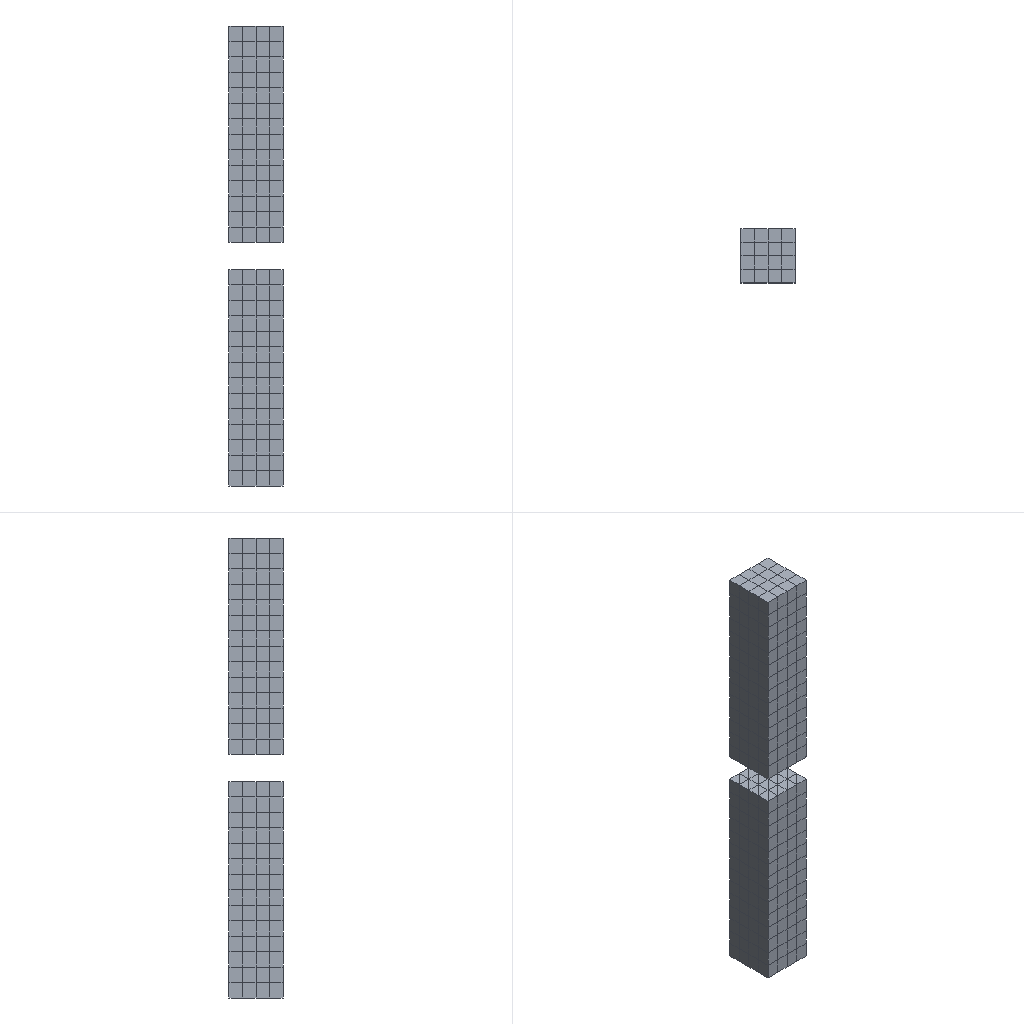Simulation study | ansys workbench
Set-up summary:
category,name,step,type,value,unit,region
solver,ansys_mapdl
solver,version,,,16.0
solver,version,,,16.0
units,MPA,,stated
analysis,deck1,,transient,transient
load_step,requested,,,1
analysis,nlgeom,,,True
mesh,nodes,,,2650
mesh,elements,,,512
element_type,ANSYS 186 (type 1),,solid,224
element_type,ANSYS 186 (type 2),,solid,224
element_type,ANSYS 174 (type 3),,contact,32
element_type,ANSYS 170 (type 4),,target,32
load,load commands in deck,,count,1
bc,support commands in deck,,count,4
named_set,_CM37UZ_ZP,,component
named_set,_DISPZEROUX,,component
named_set,_DISPZEROUY,,component
named_set,_FIXEDSU,,component
analysis,deck2,,transient,transient
load_step,requested,,,1
analysis,nlgeom,,,True
mesh,nodes,,,2650
mesh,elements,,,512
element_type,ANSYS 186 (type 1),,solid,224
element_type,ANSYS 186 (type 2),,solid,224
element_type,ANSYS 174 (type 3),,contact,32
element_type,ANSYS 170 (type 4),,target,32
load,load commands in deck,,count,1
bc,support commands in deck,,count,4
named_set,_CM37UZ_ZP,,component
named_set,_DISPZEROUX,,component
named_set,_DISPZEROUY,,component
named_set,_FIXEDSU,,component
material,1,,in results
material,2,,in results
material,1,,in results
material,2,,in results
check,setup vs results,,match
check,setup vs results,,match
Results summary:
result,analysis,,,static
result,last_loadstep,,,1
result,primary field,,,displacement
result,reaction total,10,FX,0.000214,N
result,reaction total,10,FY,0.000357,N
result,reaction total,10,FZ,-13515.283,N
result,mass,,,6.3e-05,"NMM: mm, ton, N, s, mV, mA, degC"
result,analysis,,,static
result,last_loadstep,,,1
result,primary field,,,displacement
result,reaction total,10,FX,6.3e-05,N
result,reaction total,10,FY,-2.8e-05,N
result,reaction total,10,FZ,-708.142,N
result,mass,,,6.3e-05,"NMM: mm, ton, N, s, mV, mA, degC"